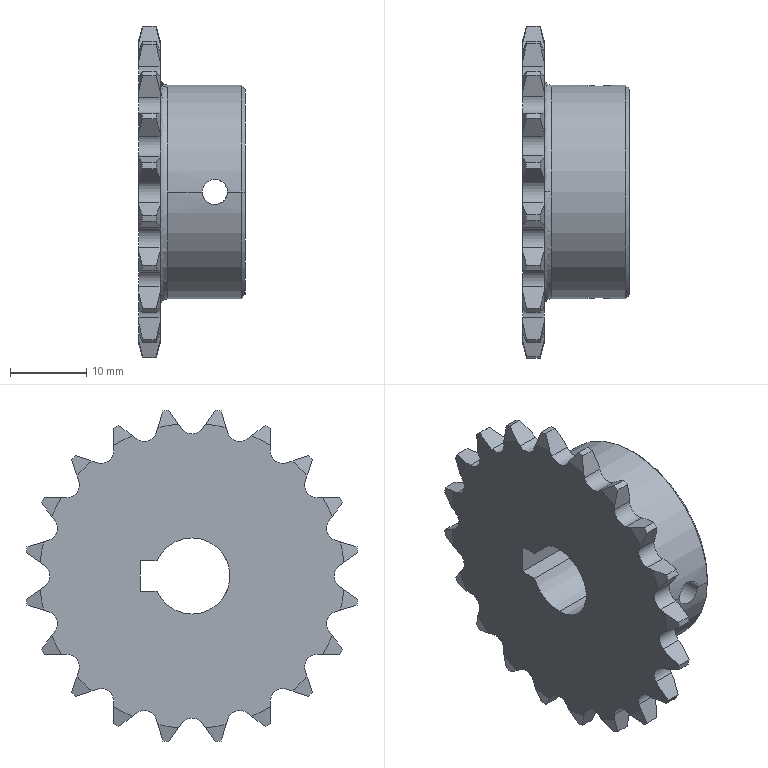Part | STEP file | 02-09 Motor sprocket | 1 solid | 146 faces | box 14 x 43.574 x 43.574 mm | volume 9063 mm3 | cylinder 56 | plane 46 | cone 42 | spline 2 | commonest cylinder face diameters 3.3 x31 44 x20 10 x3 28 x2